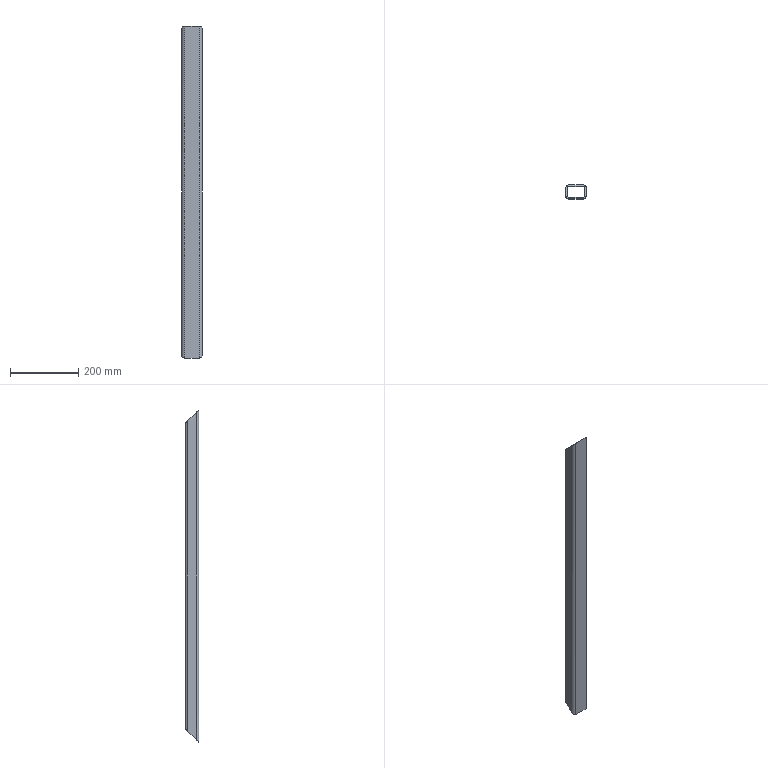Part | SolidWorks | features BaseBody 1 | 1 solid | 18 faces | box 60 x 40 x 976 mm | volume 650329 mm3 | plane 10 | cylinder 8 | commonest cylinder face diameters 8 x4 16 x4
STEP:
#1=CARTESIAN_POINT('',(-22.,-20.,976.));
#2=VERTEX_POINT('',#1);
#3=CARTESIAN_POINT('',(-22.,-20.,0.));
#4=VERTEX_POINT('',#3);
#5=CARTESIAN_POINT('',(-22.,-20.,0.));
#6=DIRECTION('',(0.,0.,-1.));
#7=VECTOR('',#6,1000.);
#8=LINE('',#5,#7);
#9=EDGE_CURVE('',#2,#4,#8,.T.);
#10=ORIENTED_EDGE('',*,*,#9,.T.);
#11=CARTESIAN_POINT('',(22.,-20.,0.));
#12=VERTEX_POINT('',#11);
#13=CARTESIAN_POINT('',(-22.,-20.,0.));
#14=DIRECTION('',(1.,0.,0.));
#15=VECTOR('',#14,1000.);
#16=LINE('',#13,#15);
#17=EDGE_CURVE('',#4,#12,#16,.T.);
#18=ORIENTED_EDGE('',*,*,#17,.T.);
#19=CARTESIAN_POINT('',(22.,-20.,976.));
#20=VERTEX_POINT('',#19);
#21=CARTESIAN_POINT('',(22.,-20.,0.));
#22=DIRECTION('',(0.,0.,1.));
#23=VECTOR('',#22,1000.);
#24=LINE('',#21,#23);
#25=EDGE_CURVE('',#12,#20,#24,.T.);
#26=ORIENTED_EDGE('',*,*,#25,.T.);
#27=CARTESIAN_POINT('',(-22.,-20.,976.));
#28=DIRECTION('',(-1.,0.,0.));
#29=VECTOR('',#28,1000.);
#30=LINE('',#27,#29);
#31=EDGE_CURVE('',#20,#2,#30,.T.);
#32=ORIENTED_EDGE('',*,*,#31,.T.);
#33=EDGE_LOOP('',(#10,#18,#26,#32));
#34=FACE_OUTER_BOUND('',#33,.T.);
#35=CARTESIAN_POINT('',(-22.,-20.,0.));
#36=DIRECTION('',(0.,-1.,0.));
#37=DIRECTION('',(0.,0.,-1.));
#38=AXIS2_PLACEMENT_3D('',#35,#36,#37);
#39=PLANE('',#38);
#40=ADVANCED_FACE('',(#34),#39,.T.);
#41=CARTESIAN_POINT('',(-26.,-12.,8.));
#42=VERTEX_POINT('',#41);
#43=CARTESIAN_POINT('',(-26.,12.,32.));
#44=VERTEX_POINT('',#43);
#45=CARTESIAN_POINT('',(-26.,-20.,0.));
#46=DIRECTION('',(0.,0.7071,0.7071));
#47=VECTOR('',#46,1000.);
#48=LINE('',#45,#47);
#49=EDGE_CURVE('',#42,#44,#48,.T.);
#50=ORIENTED_EDGE('',*,*,#49,.F.);
#51=CARTESIAN_POINT('',(-22.,-16.,4.));
#52=VERTEX_POINT('',#51);
#53=CARTESIAN_POINT('',(-22.,-16.,4.));
#54=CARTESIAN_POINT('',(-24.343,-16.,4.));
#55=CARTESIAN_POINT('',(-26.,-14.343,5.657));
#56=CARTESIAN_POINT('',(-26.,-12.,8.));
#57=(BOUNDED_CURVE()B_SPLINE_CURVE(3,(#53,#54,#55,#56),.UNSPECIFIED.,.F.,.F.)B_SPLINE_CURVE_WITH_KNOTS((4,4),(3.142,4.712),.UNSPECIFIED.)CURVE()GEOMETRIC_REPRESENTATION_ITEM()RATIONAL_B_SPLINE_CURVE((1.,0.8047,0.8047,1.))REPRESENTATION_ITEM(''));
#58=EDGE_CURVE('',#52,#42,#57,.T.);
#59=ORIENTED_EDGE('',*,*,#58,.F.);
#60=CARTESIAN_POINT('',(22.,-16.,4.));
#61=VERTEX_POINT('',#60);
#62=CARTESIAN_POINT('',(-11.546,-16.,4.));
#63=DIRECTION('',(-1.,0.,0.));
#64=VECTOR('',#63,1000.);
#65=LINE('',#62,#64);
#66=EDGE_CURVE('',#61,#52,#65,.T.);
#67=ORIENTED_EDGE('',*,*,#66,.F.);
#68=CARTESIAN_POINT('',(26.,-12.,8.));
#69=VERTEX_POINT('',#68);
#70=CARTESIAN_POINT('',(26.,-12.,8.));
#71=CARTESIAN_POINT('',(26.,-14.343,5.657));
#72=CARTESIAN_POINT('',(24.343,-16.,4.));
#73=CARTESIAN_POINT('',(22.,-16.,4.));
#74=(BOUNDED_CURVE()B_SPLINE_CURVE(3,(#70,#71,#72,#73),.UNSPECIFIED.,.F.,.T.)B_SPLINE_CURVE_WITH_KNOTS((4,4),(1.571,3.142),.UNSPECIFIED.)CURVE()GEOMETRIC_REPRESENTATION_ITEM()RATIONAL_B_SPLINE_CURVE((1.,0.8047,0.8047,1.))REPRESENTATION_ITEM(''));
#75=EDGE_CURVE('',#69,#61,#74,.T.);
#76=ORIENTED_EDGE('',*,*,#75,.F.);
#77=CARTESIAN_POINT('',(26.,12.,32.));
#78=VERTEX_POINT('',#77);
#79=CARTESIAN_POINT('',(26.,-20.,0.));
#80=DIRECTION('',(0.,-0.7071,-0.7071));
#81=VECTOR('',#80,1000.);
#82=LINE('',#79,#81);
#83=EDGE_CURVE('',#78,#69,#82,.T.);
#84=ORIENTED_EDGE('',*,*,#83,.F.);
#85=CARTESIAN_POINT('',(22.,16.,36.));
#86=VERTEX_POINT('',#85);
#87=CARTESIAN_POINT('',(22.,16.,36.));
#88=CARTESIAN_POINT('',(24.343,16.,36.));
#89=CARTESIAN_POINT('',(26.,14.343,34.343));
#90=CARTESIAN_POINT('',(26.,12.,32.));
#91=(BOUNDED_CURVE()B_SPLINE_CURVE(3,(#87,#88,#89,#90),.UNSPECIFIED.,.F.,.F.)B_SPLINE_CURVE_WITH_KNOTS((4,4),(0.,1.571),.UNSPECIFIED.)CURVE()GEOMETRIC_REPRESENTATION_ITEM()RATIONAL_B_SPLINE_CURVE((1.,0.8047,0.8047,1.))REPRESENTATION_ITEM(''));
#92=EDGE_CURVE('',#86,#78,#91,.T.);
#93=ORIENTED_EDGE('',*,*,#92,.F.);
#94=CARTESIAN_POINT('',(-22.,16.,36.));
#95=VERTEX_POINT('',#94);
#96=CARTESIAN_POINT('',(-11.546,16.,36.));
#97=DIRECTION('',(1.,0.,0.));
#98=VECTOR('',#97,1000.);
#99=LINE('',#96,#98);
#100=EDGE_CURVE('',#95,#86,#99,.T.);
#101=ORIENTED_EDGE('',*,*,#100,.F.);
#102=CARTESIAN_POINT('',(-26.,12.,32.));
#103=CARTESIAN_POINT('',(-26.,14.343,34.343));
#104=CARTESIAN_POINT('',(-24.343,16.,36.));
#105=CARTESIAN_POINT('',(-22.,16.,36.));
#106=(BOUNDED_CURVE()B_SPLINE_CURVE(3,(#102,#103,#104,#105),.UNSPECIFIED.,.F.,.F.)B_SPLINE_CURVE_WITH_KNOTS((4,4),(4.712,6.283),.UNSPECIFIED.)CURVE()GEOMETRIC_REPRESENTATION_ITEM()RATIONAL_B_SPLINE_CURVE((1.,0.8047,0.8047,1.))REPRESENTATION_ITEM(''));
#107=EDGE_CURVE('',#44,#95,#106,.T.);
#108=ORIENTED_EDGE('',*,*,#107,.F.);
#109=EDGE_LOOP('',(#50,#59,#67,#76,#84,#93,#101,#108));
#110=FACE_BOUND('',#109,.T.);
#111=CARTESIAN_POINT('',(-30.,12.,32.));
#112=VERTEX_POINT('',#111);
#113=CARTESIAN_POINT('',(-30.,-12.,8.));
#114=VERTEX_POINT('',#113);
#115=CARTESIAN_POINT('',(-30.,-20.,0.));
#116=DIRECTION('',(0.,-0.7071,-0.7071));
#117=VECTOR('',#116,1000.);
#118=LINE('',#115,#117);
#119=EDGE_CURVE('',#112,#114,#118,.T.);
#120=ORIENTED_EDGE('',*,*,#119,.F.);
#121=CARTESIAN_POINT('',(-22.,20.,40.));
#122=VERTEX_POINT('',#121);
#123=CARTESIAN_POINT('',(-22.,20.,40.));
#124=CARTESIAN_POINT('',(-26.686,20.,40.));
#125=CARTESIAN_POINT('',(-30.,16.686,36.686));
#126=CARTESIAN_POINT('',(-30.,12.,32.));
#127=(BOUNDED_CURVE()B_SPLINE_CURVE(3,(#123,#124,#125,#126),.UNSPECIFIED.,.F.,.F.)B_SPLINE_CURVE_WITH_KNOTS((4,4),(0.,1.571),.UNSPECIFIED.)CURVE()GEOMETRIC_REPRESENTATION_ITEM()RATIONAL_B_SPLINE_CURVE((1.,0.8047,0.8047,1.))REPRESENTATION_ITEM(''));
#128=EDGE_CURVE('',#122,#112,#127,.T.);
#129=ORIENTED_EDGE('',*,*,#128,.F.);
#130=CARTESIAN_POINT('',(22.,20.,40.));
#131=VERTEX_POINT('',#130);
#132=CARTESIAN_POINT('',(-11.546,20.,40.));
#133=DIRECTION('',(-1.,0.,0.));
#134=VECTOR('',#133,1000.);
#135=LINE('',#132,#134);
#136=EDGE_CURVE('',#131,#122,#135,.T.);
#137=ORIENTED_EDGE('',*,*,#136,.F.);
#138=CARTESIAN_POINT('',(30.,12.,32.));
#139=VERTEX_POINT('',#138);
#140=CARTESIAN_POINT('',(30.,12.,32.));
#141=CARTESIAN_POINT('',(30.,16.686,36.686));
#142=CARTESIAN_POINT('',(26.686,20.,40.));
#143=CARTESIAN_POINT('',(22.,20.,40.));
#144=(BOUNDED_CURVE()B_SPLINE_CURVE(3,(#140,#141,#142,#143),.UNSPECIFIED.,.F.,.F.)B_SPLINE_CURVE_WITH_KNOTS((4,4),(4.712,6.283),.UNSPECIFIED.)CURVE()GEOMETRIC_REPRESENTATION_ITEM()RATIONAL_B_SPLINE_CURVE((1.,0.8047,0.8047,1.))REPRESENTATION_ITEM(''));
#145=EDGE_CURVE('',#139,#131,#144,.T.);
#146=ORIENTED_EDGE('',*,*,#145,.F.);
#147=CARTESIAN_POINT('',(30.,-12.,8.));
#148=VERTEX_POINT('',#147);
#149=CARTESIAN_POINT('',(30.,-20.,0.));
#150=DIRECTION('',(0.,0.7071,0.7071));
#151=VECTOR('',#150,1000.);
#152=LINE('',#149,#151);
#153=EDGE_CURVE('',#148,#139,#152,.T.);
#154=ORIENTED_EDGE('',*,*,#153,.F.);
#155=CARTESIAN_POINT('',(22.,-20.,0.));
#156=CARTESIAN_POINT('',(26.686,-20.,0.));
#157=CARTESIAN_POINT('',(30.,-16.686,3.314));
#158=CARTESIAN_POINT('',(30.,-12.,8.));
#159=(BOUNDED_CURVE()B_SPLINE_CURVE(3,(#155,#156,#157,#158),.UNSPECIFIED.,.F.,.T.)B_SPLINE_CURVE_WITH_KNOTS((4,4),(3.142,4.712),.UNSPECIFIED.)CURVE()GEOMETRIC_REPRESENTATION_ITEM()RATIONAL_B_SPLINE_CURVE((1.,0.8047,0.8047,1.))REPRESENTATION_ITEM(''));
#160=EDGE_CURVE('',#12,#148,#159,.T.);
#161=ORIENTED_EDGE('',*,*,#160,.F.);
#162=ORIENTED_EDGE('',*,*,#17,.F.);
#163=CARTESIAN_POINT('',(-30.,-12.,8.));
#164=CARTESIAN_POINT('',(-30.,-16.686,3.314));
#165=CARTESIAN_POINT('',(-26.686,-20.,0.));
#166=CARTESIAN_POINT('',(-22.,-20.,0.));
#167=(BOUNDED_CURVE()B_SPLINE_CURVE(3,(#163,#164,#165,#166),.UNSPECIFIED.,.F.,.F.)B_SPLINE_CURVE_WITH_KNOTS((4,4),(1.571,3.142),.UNSPECIFIED.)CURVE()GEOMETRIC_REPRESENTATION_ITEM()RATIONAL_B_SPLINE_CURVE((1.,0.8047,0.8047,1.))REPRESENTATION_ITEM(''));
#168=EDGE_CURVE('',#114,#4,#167,.T.);
#169=ORIENTED_EDGE('',*,*,#168,.F.);
#170=EDGE_LOOP('',(#120,#129,#137,#146,#154,#161,#162,#169));
#171=FACE_OUTER_BOUND('',#170,.T.);
#172=CARTESIAN_POINT('',(-11.546,-20.,0.));
#173=DIRECTION('',(0.,-0.7071,0.7071));
#174=DIRECTION('',(0.,-0.7071,-0.7071));
#175=AXIS2_PLACEMENT_3D('',#172,#173,#174);
#176=PLANE('',#175);
#177=ADVANCED_FACE('',(#110,#171),#176,.F.);
#178=CARTESIAN_POINT('',(-30.,-12.,968.));
#179=VERTEX_POINT('',#178);
#180=CARTESIAN_POINT('',(-30.,-12.,0.));
#181=DIRECTION('',(0.,0.,-1.));
#182=VECTOR('',#181,1000.);
#183=LINE('',#180,#182);
#184=EDGE_CURVE('',#179,#114,#183,.T.);
#185=ORIENTED_EDGE('',*,*,#184,.T.);
#186=ORIENTED_EDGE('',*,*,#168,.T.);
#187=ORIENTED_EDGE('',*,*,#9,.F.);
#188=CARTESIAN_POINT('',(-22.,-20.,976.));
#189=CARTESIAN_POINT('',(-26.686,-20.,976.));
#190=CARTESIAN_POINT('',(-30.,-16.686,972.686));
#191=CARTESIAN_POINT('',(-30.,-12.,968.));
#192=(BOUNDED_CURVE()B_SPLINE_CURVE(3,(#188,#189,#190,#191),.UNSPECIFIED.,.F.,.F.)B_SPLINE_CURVE_WITH_KNOTS((4,4),(0.,1.571),.UNSPECIFIED.)CURVE()GEOMETRIC_REPRESENTATION_ITEM()RATIONAL_B_SPLINE_CURVE((1.,0.8047,0.8047,1.))REPRESENTATION_ITEM(''));
#193=EDGE_CURVE('',#2,#179,#192,.T.);
#194=ORIENTED_EDGE('',*,*,#193,.T.);
#195=EDGE_LOOP('',(#185,#186,#187,#194));
#196=FACE_OUTER_BOUND('',#195,.T.);
#197=CARTESIAN_POINT('',(-22.,-12.,0.));
#198=DIRECTION('',(0.,0.,1.));
#199=DIRECTION('',(1.,0.,0.));
#200=AXIS2_PLACEMENT_3D('',#197,#198,#199);
#201=CYLINDRICAL_SURFACE('',#200,8.);
#202=ADVANCED_FACE('',(#196),#201,.T.);
#203=CARTESIAN_POINT('',(-26.,12.,944.));
#204=VERTEX_POINT('',#203);
#205=CARTESIAN_POINT('',(-22.,16.,940.));
#206=VERTEX_POINT('',#205);
#207=CARTESIAN_POINT('',(-26.,12.,944.));
#208=CARTESIAN_POINT('',(-26.,14.343,941.657));
#209=CARTESIAN_POINT('',(-24.343,16.,940.));
#210=CARTESIAN_POINT('',(-22.,16.,940.));
#211=(BOUNDED_CURVE()B_SPLINE_CURVE(3,(#207,#208,#209,#210),.UNSPECIFIED.,.F.,.F.)B_SPLINE_CURVE_WITH_KNOTS((4,4),(1.571,3.142),.UNSPECIFIED.)CURVE()GEOMETRIC_REPRESENTATION_ITEM()RATIONAL_B_SPLINE_CURVE((1.,0.8047,0.8047,1.))REPRESENTATION_ITEM(''));
#212=EDGE_CURVE('',#204,#206,#211,.T.);
#213=ORIENTED_EDGE('',*,*,#212,.T.);
#214=CARTESIAN_POINT('',(22.,16.,940.));
#215=VERTEX_POINT('',#214);
#216=CARTESIAN_POINT('',(-11.546,16.,940.));
#217=DIRECTION('',(1.,0.,0.));
#218=VECTOR('',#217,1000.);
#219=LINE('',#216,#218);
#220=EDGE_CURVE('',#206,#215,#219,.T.);
#221=ORIENTED_EDGE('',*,*,#220,.T.);
#222=CARTESIAN_POINT('',(26.,12.,944.));
#223=VERTEX_POINT('',#222);
#224=CARTESIAN_POINT('',(22.,16.,940.));
#225=CARTESIAN_POINT('',(24.343,16.,940.));
#226=CARTESIAN_POINT('',(26.,14.343,941.657));
#227=CARTESIAN_POINT('',(26.,12.,944.));
#228=(BOUNDED_CURVE()B_SPLINE_CURVE(3,(#224,#225,#226,#227),.UNSPECIFIED.,.F.,.F.)B_SPLINE_CURVE_WITH_KNOTS((4,4),(3.142,4.712),.UNSPECIFIED.)CURVE()GEOMETRIC_REPRESENTATION_ITEM()RATIONAL_B_SPLINE_CURVE((1.,0.8047,0.8047,1.))REPRESENTATION_ITEM(''));
#229=EDGE_CURVE('',#215,#223,#228,.T.);
#230=ORIENTED_EDGE('',*,*,#229,.T.);
#231=CARTESIAN_POINT('',(26.,-12.,968.));
#232=VERTEX_POINT('',#231);
#233=CARTESIAN_POINT('',(26.,-20.,976.));
#234=DIRECTION('',(0.,-0.7071,0.7071));
#235=VECTOR('',#234,1000.);
#236=LINE('',#233,#235);
#237=EDGE_CURVE('',#223,#232,#236,.T.);
#238=ORIENTED_EDGE('',*,*,#237,.T.);
#239=CARTESIAN_POINT('',(22.,-16.,972.));
#240=VERTEX_POINT('',#239);
#241=CARTESIAN_POINT('',(26.,-12.,968.));
#242=CARTESIAN_POINT('',(26.,-14.343,970.343));
#243=CARTESIAN_POINT('',(24.343,-16.,972.));
#244=CARTESIAN_POINT('',(22.,-16.,972.));
#245=(BOUNDED_CURVE()B_SPLINE_CURVE(3,(#241,#242,#243,#244),.UNSPECIFIED.,.F.,.F.)B_SPLINE_CURVE_WITH_KNOTS((4,4),(4.712,6.283),.UNSPECIFIED.)CURVE()GEOMETRIC_REPRESENTATION_ITEM()RATIONAL_B_SPLINE_CURVE((1.,0.8047,0.8047,1.))REPRESENTATION_ITEM(''));
#246=EDGE_CURVE('',#232,#240,#245,.T.);
#247=ORIENTED_EDGE('',*,*,#246,.T.);
#248=CARTESIAN_POINT('',(-22.,-16.,972.));
#249=VERTEX_POINT('',#248);
#250=CARTESIAN_POINT('',(-11.546,-16.,972.));
#251=DIRECTION('',(-1.,0.,0.));
#252=VECTOR('',#251,1000.);
#253=LINE('',#250,#252);
#254=EDGE_CURVE('',#240,#249,#253,.T.);
#255=ORIENTED_EDGE('',*,*,#254,.T.);
#256=CARTESIAN_POINT('',(-26.,-12.,968.));
#257=VERTEX_POINT('',#256);
#258=CARTESIAN_POINT('',(-22.,-16.,972.));
#259=CARTESIAN_POINT('',(-24.343,-16.,972.));
#260=CARTESIAN_POINT('',(-26.,-14.343,970.343));
#261=CARTESIAN_POINT('',(-26.,-12.,968.));
#262=(BOUNDED_CURVE()B_SPLINE_CURVE(3,(#258,#259,#260,#261),.UNSPECIFIED.,.F.,.F.)B_SPLINE_CURVE_WITH_KNOTS((4,4),(0.,1.571),.UNSPECIFIED.)CURVE()GEOMETRIC_REPRESENTATION_ITEM()RATIONAL_B_SPLINE_CURVE((1.,0.8047,0.8047,1.))REPRESENTATION_ITEM(''));
#263=EDGE_CURVE('',#249,#257,#262,.T.);
#264=ORIENTED_EDGE('',*,*,#263,.T.);
#265=CARTESIAN_POINT('',(-26.,-20.,976.));
#266=DIRECTION('',(0.,0.7071,-0.7071));
#267=VECTOR('',#266,1000.);
#268=LINE('',#265,#267);
#269=EDGE_CURVE('',#257,#204,#268,.T.);
#270=ORIENTED_EDGE('',*,*,#269,.T.);
#271=EDGE_LOOP('',(#213,#221,#230,#238,#247,#255,#264,#270));
#272=FACE_BOUND('',#271,.T.);
#273=ORIENTED_EDGE('',*,*,#193,.F.);
#274=ORIENTED_EDGE('',*,*,#31,.F.);
#275=CARTESIAN_POINT('',(30.,-12.,968.));
#276=VERTEX_POINT('',#275);
#277=CARTESIAN_POINT('',(22.,-20.,976.));
#278=CARTESIAN_POINT('',(26.686,-20.,976.));
#279=CARTESIAN_POINT('',(30.,-16.686,972.686));
#280=CARTESIAN_POINT('',(30.,-12.,968.));
#281=(BOUNDED_CURVE()B_SPLINE_CURVE(3,(#277,#278,#279,#280),.UNSPECIFIED.,.F.,.F.)B_SPLINE_CURVE_WITH_KNOTS((4,4),(0.,1.571),.UNSPECIFIED.)CURVE()GEOMETRIC_REPRESENTATION_ITEM()RATIONAL_B_SPLINE_CURVE((1.,0.8047,0.8047,1.))REPRESENTATION_ITEM(''));
#282=EDGE_CURVE('',#20,#276,#281,.T.);
#283=ORIENTED_EDGE('',*,*,#282,.T.);
#284=CARTESIAN_POINT('',(30.,12.,944.));
#285=VERTEX_POINT('',#284);
#286=CARTESIAN_POINT('',(30.,-20.,976.));
#287=DIRECTION('',(0.,0.7071,-0.7071));
#288=VECTOR('',#287,1000.);
#289=LINE('',#286,#288);
#290=EDGE_CURVE('',#276,#285,#289,.T.);
#291=ORIENTED_EDGE('',*,*,#290,.T.);
#292=CARTESIAN_POINT('',(22.,20.,936.));
#293=VERTEX_POINT('',#292);
#294=CARTESIAN_POINT('',(30.,12.,944.));
#295=CARTESIAN_POINT('',(30.,16.686,939.314));
#296=CARTESIAN_POINT('',(26.686,20.,936.));
#297=CARTESIAN_POINT('',(22.,20.,936.));
#298=(BOUNDED_CURVE()B_SPLINE_CURVE(3,(#294,#295,#296,#297),.UNSPECIFIED.,.F.,.F.)B_SPLINE_CURVE_WITH_KNOTS((4,4),(1.571,3.142),.UNSPECIFIED.)CURVE()GEOMETRIC_REPRESENTATION_ITEM()RATIONAL_B_SPLINE_CURVE((1.,0.8047,0.8047,1.))REPRESENTATION_ITEM(''));
#299=EDGE_CURVE('',#285,#293,#298,.T.);
#300=ORIENTED_EDGE('',*,*,#299,.T.);
#301=CARTESIAN_POINT('',(-22.,20.,936.));
#302=VERTEX_POINT('',#301);
#303=CARTESIAN_POINT('',(-11.546,20.,936.));
#304=DIRECTION('',(-1.,0.,0.));
#305=VECTOR('',#304,1000.);
#306=LINE('',#303,#305);
#307=EDGE_CURVE('',#293,#302,#306,.T.);
#308=ORIENTED_EDGE('',*,*,#307,.T.);
#309=CARTESIAN_POINT('',(-30.,12.,944.));
#310=VERTEX_POINT('',#309);
#311=CARTESIAN_POINT('',(-22.,20.,936.));
#312=CARTESIAN_POINT('',(-26.686,20.,936.));
#313=CARTESIAN_POINT('',(-30.,16.686,939.314));
#314=CARTESIAN_POINT('',(-30.,12.,944.));
#315=(BOUNDED_CURVE()B_SPLINE_CURVE(3,(#311,#312,#313,#314),.UNSPECIFIED.,.F.,.F.)B_SPLINE_CURVE_WITH_KNOTS((4,4),(3.142,4.712),.UNSPECIFIED.)CURVE()GEOMETRIC_REPRESENTATION_ITEM()RATIONAL_B_SPLINE_CURVE((1.,0.8047,0.8047,1.))REPRESENTATION_ITEM(''));
#316=EDGE_CURVE('',#302,#310,#315,.T.);
#317=ORIENTED_EDGE('',*,*,#316,.T.);
#318=CARTESIAN_POINT('',(-30.,-20.,976.));
#319=DIRECTION('',(0.,-0.7071,0.7071));
#320=VECTOR('',#319,1000.);
#321=LINE('',#318,#320);
#322=EDGE_CURVE('',#310,#179,#321,.T.);
#323=ORIENTED_EDGE('',*,*,#322,.T.);
#324=EDGE_LOOP('',(#273,#274,#283,#291,#300,#308,#317,#323));
#325=FACE_OUTER_BOUND('',#324,.T.);
#326=CARTESIAN_POINT('',(-11.546,-20.,976.));
#327=DIRECTION('',(0.,0.7071,0.7071));
#328=DIRECTION('',(0.,-0.7071,0.7071));
#329=AXIS2_PLACEMENT_3D('',#326,#327,#328);
#330=PLANE('',#329);
#331=ADVANCED_FACE('',(#272,#325),#330,.T.);
#332=ORIENTED_EDGE('',*,*,#25,.F.);
#333=ORIENTED_EDGE('',*,*,#160,.T.);
#334=CARTESIAN_POINT('',(30.,-12.,0.));
#335=DIRECTION('',(0.,0.,1.));
#336=VECTOR('',#335,1000.);
#337=LINE('',#334,#336);
#338=EDGE_CURVE('',#148,#276,#337,.T.);
#339=ORIENTED_EDGE('',*,*,#338,.T.);
#340=ORIENTED_EDGE('',*,*,#282,.F.);
#341=EDGE_LOOP('',(#332,#333,#339,#340));
#342=FACE_OUTER_BOUND('',#341,.T.);
#343=CARTESIAN_POINT('',(22.,-12.,0.));
#344=DIRECTION('',(0.,0.,1.));
#345=DIRECTION('',(1.,0.,0.));
#346=AXIS2_PLACEMENT_3D('',#343,#344,#345);
#347=CYLINDRICAL_SURFACE('',#346,8.);
#348=ADVANCED_FACE('',(#342),#347,.T.);
#349=ORIENTED_EDGE('',*,*,#212,.F.);
#350=CARTESIAN_POINT('',(-26.,12.,0.));
#351=DIRECTION('',(0.,0.,1.));
#352=VECTOR('',#351,1000.);
#353=LINE('',#350,#352);
#354=EDGE_CURVE('',#44,#204,#353,.T.);
#355=ORIENTED_EDGE('',*,*,#354,.F.);
#356=ORIENTED_EDGE('',*,*,#107,.T.);
#357=CARTESIAN_POINT('',(-22.,16.,0.));
#358=DIRECTION('',(0.,0.,-1.));
#359=VECTOR('',#358,1000.);
#360=LINE('',#357,#359);
#361=EDGE_CURVE('',#206,#95,#360,.T.);
#362=ORIENTED_EDGE('',*,*,#361,.F.);
#363=EDGE_LOOP('',(#349,#355,#356,#362));
#364=FACE_OUTER_BOUND('',#363,.T.);
#365=CARTESIAN_POINT('',(-22.,12.,0.));
#366=DIRECTION('',(0.,0.,1.));
#367=DIRECTION('',(1.,0.,0.));
#368=AXIS2_PLACEMENT_3D('',#365,#366,#367);
#369=CYLINDRICAL_SURFACE('',#368,4.);
#370=ADVANCED_FACE('',(#364),#369,.F.);
#371=CARTESIAN_POINT('',(-26.,-12.,0.));
#372=DIRECTION('',(0.,0.,-1.));
#373=VECTOR('',#372,1000.);
#374=LINE('',#371,#373);
#375=EDGE_CURVE('',#257,#42,#374,.T.);
#376=ORIENTED_EDGE('',*,*,#375,.T.);
#377=ORIENTED_EDGE('',*,*,#49,.T.);
#378=ORIENTED_EDGE('',*,*,#354,.T.);
#379=ORIENTED_EDGE('',*,*,#269,.F.);
#380=EDGE_LOOP('',(#376,#377,#378,#379));
#381=FACE_OUTER_BOUND('',#380,.T.);
#382=CARTESIAN_POINT('',(-26.,-12.,0.));
#383=DIRECTION('',(1.,0.,0.));
#384=DIRECTION('',(0.,0.,-1.));
#385=AXIS2_PLACEMENT_3D('',#382,#383,#384);
#386=PLANE('',#385);
#387=ADVANCED_FACE('',(#381),#386,.T.);
#388=ORIENTED_EDGE('',*,*,#263,.F.);
#389=CARTESIAN_POINT('',(-22.,-16.,0.));
#390=DIRECTION('',(0.,0.,1.));
#391=VECTOR('',#390,1000.);
#392=LINE('',#389,#391);
#393=EDGE_CURVE('',#52,#249,#392,.T.);
#394=ORIENTED_EDGE('',*,*,#393,.F.);
#395=ORIENTED_EDGE('',*,*,#58,.T.);
#396=ORIENTED_EDGE('',*,*,#375,.F.);
#397=EDGE_LOOP('',(#388,#394,#395,#396));
#398=FACE_OUTER_BOUND('',#397,.T.);
#399=CARTESIAN_POINT('',(-22.,-12.,0.));
#400=DIRECTION('',(0.,0.,1.));
#401=DIRECTION('',(1.,0.,0.));
#402=AXIS2_PLACEMENT_3D('',#399,#400,#401);
#403=CYLINDRICAL_SURFACE('',#402,4.);
#404=ADVANCED_FACE('',(#398),#403,.F.);
#405=CARTESIAN_POINT('',(22.,-16.,0.));
#406=DIRECTION('',(0.,0.,-1.));
#407=VECTOR('',#406,1000.);
#408=LINE('',#405,#407);
#409=EDGE_CURVE('',#240,#61,#408,.T.);
#410=ORIENTED_EDGE('',*,*,#409,.T.);
#411=ORIENTED_EDGE('',*,*,#66,.T.);
#412=ORIENTED_EDGE('',*,*,#393,.T.);
#413=ORIENTED_EDGE('',*,*,#254,.F.);
#414=EDGE_LOOP('',(#410,#411,#412,#413));
#415=FACE_OUTER_BOUND('',#414,.T.);
#416=CARTESIAN_POINT('',(22.,-16.,0.));
#417=DIRECTION('',(0.,1.,0.));
#418=DIRECTION('',(0.,0.,1.));
#419=AXIS2_PLACEMENT_3D('',#416,#417,#418);
#420=PLANE('',#419);
#421=ADVANCED_FACE('',(#415),#420,.T.);
#422=ORIENTED_EDGE('',*,*,#246,.F.);
#423=CARTESIAN_POINT('',(26.,-12.,0.));
#424=DIRECTION('',(0.,0.,1.));
#425=VECTOR('',#424,1000.);
#426=LINE('',#423,#425);
#427=EDGE_CURVE('',#69,#232,#426,.T.);
#428=ORIENTED_EDGE('',*,*,#427,.F.);
#429=ORIENTED_EDGE('',*,*,#75,.T.);
#430=ORIENTED_EDGE('',*,*,#409,.F.);
#431=EDGE_LOOP('',(#422,#428,#429,#430));
#432=FACE_OUTER_BOUND('',#431,.T.);
#433=CARTESIAN_POINT('',(22.,-12.,0.));
#434=DIRECTION('',(0.,0.,1.));
#435=DIRECTION('',(1.,0.,0.));
#436=AXIS2_PLACEMENT_3D('',#433,#434,#435);
#437=CYLINDRICAL_SURFACE('',#436,4.);
#438=ADVANCED_FACE('',(#432),#437,.F.);
#439=CARTESIAN_POINT('',(26.,12.,0.));
#440=DIRECTION('',(0.,0.,-1.));
#441=VECTOR('',#440,1000.);
#442=LINE('',#439,#441);
#443=EDGE_CURVE('',#223,#78,#442,.T.);
#444=ORIENTED_EDGE('',*,*,#443,.T.);
#445=ORIENTED_EDGE('',*,*,#83,.T.);
#446=ORIENTED_EDGE('',*,*,#427,.T.);
#447=ORIENTED_EDGE('',*,*,#237,.F.);
#448=EDGE_LOOP('',(#444,#445,#446,#447));
#449=FACE_OUTER_BOUND('',#448,.T.);
#450=CARTESIAN_POINT('',(26.,12.,0.));
#451=DIRECTION('',(-1.,0.,0.));
#452=DIRECTION('',(0.,0.,1.));
#453=AXIS2_PLACEMENT_3D('',#450,#451,#452);
#454=PLANE('',#453);
#455=ADVANCED_FACE('',(#449),#454,.T.);
#456=ORIENTED_EDGE('',*,*,#229,.F.);
#457=CARTESIAN_POINT('',(22.,16.,0.));
#458=DIRECTION('',(0.,0.,1.));
#459=VECTOR('',#458,1000.);
#460=LINE('',#457,#459);
#461=EDGE_CURVE('',#86,#215,#460,.T.);
#462=ORIENTED_EDGE('',*,*,#461,.F.);
#463=ORIENTED_EDGE('',*,*,#92,.T.);
#464=ORIENTED_EDGE('',*,*,#443,.F.);
#465=EDGE_LOOP('',(#456,#462,#463,#464));
#466=FACE_OUTER_BOUND('',#465,.T.);
#467=CARTESIAN_POINT('',(22.,12.,0.));
#468=DIRECTION('',(0.,0.,1.));
#469=DIRECTION('',(1.,0.,0.));
#470=AXIS2_PLACEMENT_3D('',#467,#468,#469);
#471=CYLINDRICAL_SURFACE('',#470,4.);
#472=ADVANCED_FACE('',(#466),#471,.F.);
#473=ORIENTED_EDGE('',*,*,#361,.T.);
#474=ORIENTED_EDGE('',*,*,#100,.T.);
#475=ORIENTED_EDGE('',*,*,#461,.T.);
#476=ORIENTED_EDGE('',*,*,#220,.F.);
#477=EDGE_LOOP('',(#473,#474,#475,#476));
#478=FACE_OUTER_BOUND('',#477,.T.);
#479=CARTESIAN_POINT('',(-22.,16.,0.));
#480=DIRECTION('',(0.,-1.,0.));
#481=DIRECTION('',(0.,0.,-1.));
#482=AXIS2_PLACEMENT_3D('',#479,#480,#481);
#483=PLANE('',#482);
#484=ADVANCED_FACE('',(#478),#483,.T.);
#485=CARTESIAN_POINT('',(-30.,12.,0.));
#486=DIRECTION('',(0.,0.,-1.));
#487=VECTOR('',#486,1000.);
#488=LINE('',#485,#487);
#489=EDGE_CURVE('',#310,#112,#488,.T.);
#490=ORIENTED_EDGE('',*,*,#489,.T.);
#491=ORIENTED_EDGE('',*,*,#119,.T.);
#492=ORIENTED_EDGE('',*,*,#184,.F.);
#493=ORIENTED_EDGE('',*,*,#322,.F.);
#494=EDGE_LOOP('',(#490,#491,#492,#493));
#495=FACE_OUTER_BOUND('',#494,.T.);
#496=CARTESIAN_POINT('',(-30.,12.,0.));
#497=DIRECTION('',(-1.,0.,0.));
#498=DIRECTION('',(0.,0.,1.));
#499=AXIS2_PLACEMENT_3D('',#496,#497,#498);
#500=PLANE('',#499);
#501=ADVANCED_FACE('',(#495),#500,.T.);
#502=CARTESIAN_POINT('',(22.,20.,0.));
#503=DIRECTION('',(0.,0.,-1.));
#504=VECTOR('',#503,1000.);
#505=LINE('',#502,#504);
#506=EDGE_CURVE('',#293,#131,#505,.T.);
#507=ORIENTED_EDGE('',*,*,#506,.T.);
#508=ORIENTED_EDGE('',*,*,#136,.T.);
#509=CARTESIAN_POINT('',(-22.,20.,0.));
#510=DIRECTION('',(0.,0.,1.));
#511=VECTOR('',#510,1000.);
#512=LINE('',#509,#511);
#513=EDGE_CURVE('',#122,#302,#512,.T.);
#514=ORIENTED_EDGE('',*,*,#513,.T.);
#515=ORIENTED_EDGE('',*,*,#307,.F.);
#516=EDGE_LOOP('',(#507,#508,#514,#515));
#517=FACE_OUTER_BOUND('',#516,.T.);
#518=CARTESIAN_POINT('',(22.,20.,0.));
#519=DIRECTION('',(0.,1.,0.));
#520=DIRECTION('',(0.,0.,1.));
#521=AXIS2_PLACEMENT_3D('',#518,#519,#520);
#522=PLANE('',#521);
#523=ADVANCED_FACE('',(#517),#522,.T.);
#524=ORIENTED_EDGE('',*,*,#338,.F.);
#525=ORIENTED_EDGE('',*,*,#153,.T.);
#526=CARTESIAN_POINT('',(30.,12.,0.));
#527=DIRECTION('',(0.,0.,1.));
#528=VECTOR('',#527,1000.);
#529=LINE('',#526,#528);
#530=EDGE_CURVE('',#139,#285,#529,.T.);
#531=ORIENTED_EDGE('',*,*,#530,.T.);
#532=ORIENTED_EDGE('',*,*,#290,.F.);
#533=EDGE_LOOP('',(#524,#525,#531,#532));
#534=FACE_OUTER_BOUND('',#533,.T.);
#535=CARTESIAN_POINT('',(30.,-12.,0.));
#536=DIRECTION('',(1.,0.,0.));
#537=DIRECTION('',(0.,0.,-1.));
#538=AXIS2_PLACEMENT_3D('',#535,#536,#537);
#539=PLANE('',#538);
#540=ADVANCED_FACE('',(#534),#539,.T.);
#541=ORIENTED_EDGE('',*,*,#513,.F.);
#542=ORIENTED_EDGE('',*,*,#128,.T.);
#543=ORIENTED_EDGE('',*,*,#489,.F.);
#544=ORIENTED_EDGE('',*,*,#316,.F.);
#545=EDGE_LOOP('',(#541,#542,#543,#544));
#546=FACE_OUTER_BOUND('',#545,.T.);
#547=CARTESIAN_POINT('',(-22.,12.,0.));
#548=DIRECTION('',(0.,0.,1.));
#549=DIRECTION('',(1.,0.,0.));
#550=AXIS2_PLACEMENT_3D('',#547,#548,#549);
#551=CYLINDRICAL_SURFACE('',#550,8.);
#552=ADVANCED_FACE('',(#546),#551,.T.);
#553=ORIENTED_EDGE('',*,*,#530,.F.);
#554=ORIENTED_EDGE('',*,*,#145,.T.);
#555=ORIENTED_EDGE('',*,*,#506,.F.);
#556=ORIENTED_EDGE('',*,*,#299,.F.);
#557=EDGE_LOOP('',(#553,#554,#555,#556));
#558=FACE_OUTER_BOUND('',#557,.T.);
#559=CARTESIAN_POINT('',(22.,12.,0.));
#560=DIRECTION('',(0.,0.,1.));
#561=DIRECTION('',(1.,0.,0.));
#562=AXIS2_PLACEMENT_3D('',#559,#560,#561);
#563=CYLINDRICAL_SURFACE('',#562,8.);
#564=ADVANCED_FACE('',(#558),#563,.T.);
#565=CLOSED_SHELL('',(#40,#177,#202,#331,#348,#370,#387,#404,#421,#438,#455,#472,#484,#501,#523,#540,#552,#564));
#566=MANIFOLD_SOLID_BREP('',#565);
#567=CARTESIAN_POINT('',(0.,0.,0.));
#568=DIRECTION('',(0.,0.,1.));
#569=DIRECTION('',(1.,0.,0.));
#570=AXIS2_PLACEMENT_3D('',#567,#568,#569);
#571=(LENGTH_UNIT()NAMED_UNIT(*)SI_UNIT(.MILLI.,.METRE.));
#572=UNCERTAINTY_MEASURE_WITH_UNIT(LENGTH_MEASURE(0.00001),#571,'','');
#573=(NAMED_UNIT(*)PLANE_ANGLE_UNIT()SI_UNIT($,.RADIAN.));
#574=(NAMED_UNIT(*)SI_UNIT($,.STERADIAN.)SOLID_ANGLE_UNIT());
#575=(GEOMETRIC_REPRESENTATION_CONTEXT(3)GLOBAL_UNCERTAINTY_ASSIGNED_CONTEXT((#572))GLOBAL_UNIT_ASSIGNED_CONTEXT((#571,#573,#574))REPRESENTATION_CONTEXT('',''));
#576=ADVANCED_BREP_SHAPE_REPRESENTATION('',(#566,#570),#575);